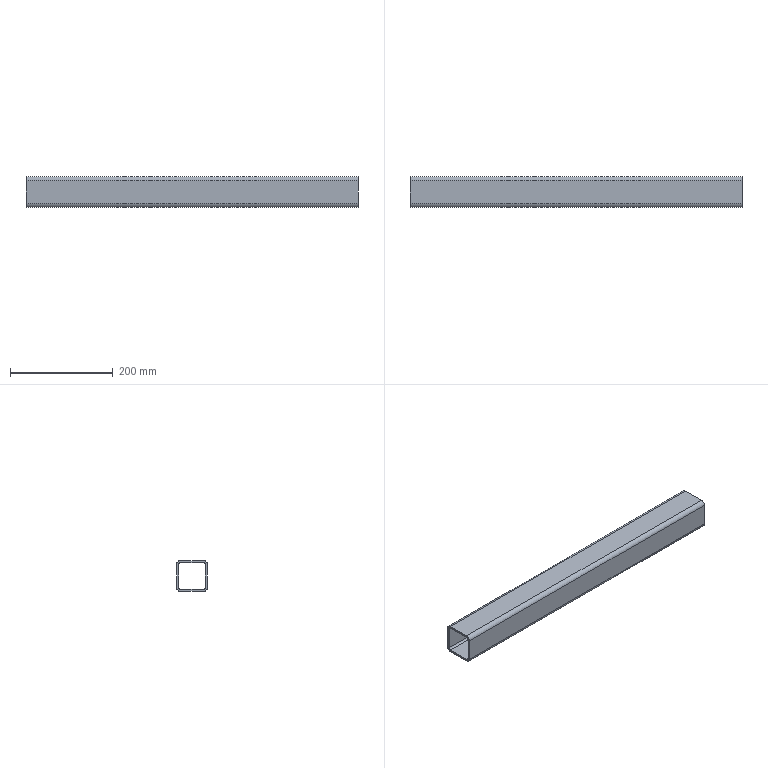Part | SolidWorks | features BaseBody 1 | 1 solid | 18 faces | box 645 x 60 x 60 mm | volume 551344 mm3 | plane 10 | cylinder 8 | commonest cylinder face diameters 8 x4 16 x4
STEP:
#1=CARTESIAN_POINT('',(700.,2488.,-1292.));
#2=VERTEX_POINT('',#1);
#3=CARTESIAN_POINT('',(700.,2488.,-1248.));
#4=VERTEX_POINT('',#3);
#5=CARTESIAN_POINT('',(700.,2488.,-1292.));
#6=DIRECTION('',(0.,0.,1.));
#7=VECTOR('',#6,1000.);
#8=LINE('',#5,#7);
#9=EDGE_CURVE('',#2,#4,#8,.T.);
#10=ORIENTED_EDGE('',*,*,#9,.T.);
#11=CARTESIAN_POINT('',(55.,2488.,-1248.));
#12=VERTEX_POINT('',#11);
#13=CARTESIAN_POINT('',(25.,2488.,-1248.));
#14=DIRECTION('',(-1.,0.,0.));
#15=VECTOR('',#14,1000.);
#16=LINE('',#13,#15);
#17=EDGE_CURVE('',#4,#12,#16,.T.);
#18=ORIENTED_EDGE('',*,*,#17,.T.);
#19=CARTESIAN_POINT('',(55.,2488.,-1292.));
#20=VERTEX_POINT('',#19);
#21=CARTESIAN_POINT('',(55.,2488.,-1292.));
#22=DIRECTION('',(0.,0.,-1.));
#23=VECTOR('',#22,1000.);
#24=LINE('',#21,#23);
#25=EDGE_CURVE('',#12,#20,#24,.T.);
#26=ORIENTED_EDGE('',*,*,#25,.T.);
#27=CARTESIAN_POINT('',(25.,2488.,-1292.));
#28=DIRECTION('',(1.,0.,0.));
#29=VECTOR('',#28,1000.);
#30=LINE('',#27,#29);
#31=EDGE_CURVE('',#20,#2,#30,.T.);
#32=ORIENTED_EDGE('',*,*,#31,.T.);
#33=EDGE_LOOP('',(#10,#18,#26,#32));
#34=FACE_OUTER_BOUND('',#33,.T.);
#35=CARTESIAN_POINT('',(25.,2488.,-1292.));
#36=DIRECTION('',(0.,-1.,0.));
#37=DIRECTION('',(0.,0.,-1.));
#38=AXIS2_PLACEMENT_3D('',#35,#36,#37);
#39=PLANE('',#38);
#40=ADVANCED_FACE('',(#34),#39,.T.);
#41=ORIENTED_EDGE('',*,*,#17,.F.);
#42=CARTESIAN_POINT('',(700.,2484.,-1244.));
#43=VERTEX_POINT('',#42);
#44=CARTESIAN_POINT('',(700.,2484.,-1248.));
#45=DIRECTION('',(-1.,0.,0.));
#46=DIRECTION('',(0.,0.,-1.));
#47=AXIS2_PLACEMENT_3D('',#44,#45,#46);
#48=CIRCLE('',#47,4.);
#49=EDGE_CURVE('',#43,#4,#48,.T.);
#50=ORIENTED_EDGE('',*,*,#49,.F.);
#51=CARTESIAN_POINT('',(55.,2484.,-1244.));
#52=VERTEX_POINT('',#51);
#53=CARTESIAN_POINT('',(25.,2484.,-1244.));
#54=DIRECTION('',(1.,0.,0.));
#55=VECTOR('',#54,1000.);
#56=LINE('',#53,#55);
#57=EDGE_CURVE('',#52,#43,#56,.T.);
#58=ORIENTED_EDGE('',*,*,#57,.F.);
#59=CARTESIAN_POINT('',(55.,2484.,-1248.));
#60=DIRECTION('',(1.,0.,0.));
#61=DIRECTION('',(0.,0.,-1.));
#62=AXIS2_PLACEMENT_3D('',#59,#60,#61);
#63=CIRCLE('',#62,4.);
#64=EDGE_CURVE('',#12,#52,#63,.T.);
#65=ORIENTED_EDGE('',*,*,#64,.F.);
#66=EDGE_LOOP('',(#41,#50,#58,#65));
#67=FACE_OUTER_BOUND('',#66,.T.);
#68=CARTESIAN_POINT('',(25.,2484.,-1248.));
#69=DIRECTION('',(1.,0.,0.));
#70=DIRECTION('',(0.,0.,-1.));
#71=AXIS2_PLACEMENT_3D('',#68,#69,#70);
#72=CYLINDRICAL_SURFACE('',#71,4.);
#73=ADVANCED_FACE('',(#67),#72,.F.);
#74=CARTESIAN_POINT('',(700.,2440.,-1244.));
#75=VERTEX_POINT('',#74);
#76=CARTESIAN_POINT('',(700.,2462.,-1244.));
#77=DIRECTION('',(0.,1.,0.));
#78=VECTOR('',#77,1000.);
#79=LINE('',#76,#78);
#80=EDGE_CURVE('',#75,#43,#79,.T.);
#81=ORIENTED_EDGE('',*,*,#80,.T.);
#82=ORIENTED_EDGE('',*,*,#49,.T.);
#83=ORIENTED_EDGE('',*,*,#9,.F.);
#84=CARTESIAN_POINT('',(700.,2484.,-1296.));
#85=VERTEX_POINT('',#84);
#86=CARTESIAN_POINT('',(700.,2484.,-1292.));
#87=DIRECTION('',(-1.,0.,0.));
#88=DIRECTION('',(0.,0.,-1.));
#89=AXIS2_PLACEMENT_3D('',#86,#87,#88);
#90=CIRCLE('',#89,4.);
#91=EDGE_CURVE('',#2,#85,#90,.T.);
#92=ORIENTED_EDGE('',*,*,#91,.T.);
#93=CARTESIAN_POINT('',(700.,2440.,-1296.));
#94=VERTEX_POINT('',#93);
#95=CARTESIAN_POINT('',(700.,2462.,-1296.));
#96=DIRECTION('',(0.,-1.,0.));
#97=VECTOR('',#96,1000.);
#98=LINE('',#95,#97);
#99=EDGE_CURVE('',#85,#94,#98,.T.);
#100=ORIENTED_EDGE('',*,*,#99,.T.);
#101=CARTESIAN_POINT('',(700.,2436.,-1292.));
#102=VERTEX_POINT('',#101);
#103=CARTESIAN_POINT('',(700.,2440.,-1292.));
#104=DIRECTION('',(-1.,0.,0.));
#105=DIRECTION('',(0.,0.,-1.));
#106=AXIS2_PLACEMENT_3D('',#103,#104,#105);
#107=CIRCLE('',#106,4.);
#108=EDGE_CURVE('',#94,#102,#107,.T.);
#109=ORIENTED_EDGE('',*,*,#108,.T.);
#110=CARTESIAN_POINT('',(700.,2436.,-1248.));
#111=VERTEX_POINT('',#110);
#112=CARTESIAN_POINT('',(700.,2436.,-1300.));
#113=DIRECTION('',(0.,0.,1.));
#114=VECTOR('',#113,1000.);
#115=LINE('',#112,#114);
#116=EDGE_CURVE('',#102,#111,#115,.T.);
#117=ORIENTED_EDGE('',*,*,#116,.T.);
#118=CARTESIAN_POINT('',(700.,2440.,-1248.));
#119=DIRECTION('',(-1.,0.,0.));
#120=DIRECTION('',(0.,0.,-1.));
#121=AXIS2_PLACEMENT_3D('',#118,#119,#120);
#122=CIRCLE('',#121,4.);
#123=EDGE_CURVE('',#111,#75,#122,.T.);
#124=ORIENTED_EDGE('',*,*,#123,.T.);
#125=EDGE_LOOP('',(#81,#82,#83,#92,#100,#109,#117,#124));
#126=FACE_BOUND('',#125,.T.);
#127=CARTESIAN_POINT('',(700.,2492.,-1248.));
#128=VERTEX_POINT('',#127);
#129=CARTESIAN_POINT('',(700.,2484.,-1240.));
#130=VERTEX_POINT('',#129);
#131=CARTESIAN_POINT('',(700.,2484.,-1248.));
#132=DIRECTION('',(1.,0.,0.));
#133=DIRECTION('',(0.,0.,-1.));
#134=AXIS2_PLACEMENT_3D('',#131,#132,#133);
#135=CIRCLE('',#134,8.);
#136=EDGE_CURVE('',#128,#130,#135,.T.);
#137=ORIENTED_EDGE('',*,*,#136,.T.);
#138=CARTESIAN_POINT('',(700.,2440.,-1240.));
#139=VERTEX_POINT('',#138);
#140=CARTESIAN_POINT('',(700.,2462.,-1240.));
#141=DIRECTION('',(0.,-1.,0.));
#142=VECTOR('',#141,1000.);
#143=LINE('',#140,#142);
#144=EDGE_CURVE('',#130,#139,#143,.T.);
#145=ORIENTED_EDGE('',*,*,#144,.T.);
#146=CARTESIAN_POINT('',(700.,2432.,-1248.));
#147=VERTEX_POINT('',#146);
#148=CARTESIAN_POINT('',(700.,2440.,-1248.));
#149=DIRECTION('',(1.,0.,0.));
#150=DIRECTION('',(0.,0.,-1.));
#151=AXIS2_PLACEMENT_3D('',#148,#149,#150);
#152=CIRCLE('',#151,8.);
#153=EDGE_CURVE('',#139,#147,#152,.T.);
#154=ORIENTED_EDGE('',*,*,#153,.T.);
#155=CARTESIAN_POINT('',(700.,2432.,-1292.));
#156=VERTEX_POINT('',#155);
#157=CARTESIAN_POINT('',(700.,2432.,-1300.));
#158=DIRECTION('',(0.,0.,-1.));
#159=VECTOR('',#158,1000.);
#160=LINE('',#157,#159);
#161=EDGE_CURVE('',#147,#156,#160,.T.);
#162=ORIENTED_EDGE('',*,*,#161,.T.);
#163=CARTESIAN_POINT('',(700.,2440.,-1300.));
#164=VERTEX_POINT('',#163);
#165=CARTESIAN_POINT('',(700.,2440.,-1292.));
#166=DIRECTION('',(1.,0.,0.));
#167=DIRECTION('',(0.,0.,-1.));
#168=AXIS2_PLACEMENT_3D('',#165,#166,#167);
#169=CIRCLE('',#168,8.);
#170=EDGE_CURVE('',#156,#164,#169,.T.);
#171=ORIENTED_EDGE('',*,*,#170,.T.);
#172=CARTESIAN_POINT('',(700.,2484.,-1300.));
#173=VERTEX_POINT('',#172);
#174=CARTESIAN_POINT('',(700.,2462.,-1300.));
#175=DIRECTION('',(0.,1.,0.));
#176=VECTOR('',#175,1000.);
#177=LINE('',#174,#176);
#178=EDGE_CURVE('',#164,#173,#177,.T.);
#179=ORIENTED_EDGE('',*,*,#178,.T.);
#180=CARTESIAN_POINT('',(700.,2492.,-1292.));
#181=VERTEX_POINT('',#180);
#182=CARTESIAN_POINT('',(700.,2484.,-1292.));
#183=DIRECTION('',(1.,0.,0.));
#184=DIRECTION('',(0.,0.,-1.));
#185=AXIS2_PLACEMENT_3D('',#182,#183,#184);
#186=CIRCLE('',#185,8.);
#187=EDGE_CURVE('',#173,#181,#186,.T.);
#188=ORIENTED_EDGE('',*,*,#187,.T.);
#189=CARTESIAN_POINT('',(700.,2492.,-1300.));
#190=DIRECTION('',(0.,0.,1.));
#191=VECTOR('',#190,1000.);
#192=LINE('',#189,#191);
#193=EDGE_CURVE('',#181,#128,#192,.T.);
#194=ORIENTED_EDGE('',*,*,#193,.T.);
#195=EDGE_LOOP('',(#137,#145,#154,#162,#171,#179,#188,#194));
#196=FACE_OUTER_BOUND('',#195,.T.);
#197=CARTESIAN_POINT('',(700.,2462.,-1300.));
#198=DIRECTION('',(1.,0.,0.));
#199=DIRECTION('',(0.,0.,-1.));
#200=AXIS2_PLACEMENT_3D('',#197,#198,#199);
#201=PLANE('',#200);
#202=ADVANCED_FACE('',(#126,#196),#201,.T.);
#203=CARTESIAN_POINT('',(55.,2484.,-1296.));
#204=VERTEX_POINT('',#203);
#205=CARTESIAN_POINT('',(25.,2484.,-1296.));
#206=DIRECTION('',(-1.,0.,0.));
#207=VECTOR('',#206,1000.);
#208=LINE('',#205,#207);
#209=EDGE_CURVE('',#85,#204,#208,.T.);
#210=ORIENTED_EDGE('',*,*,#209,.F.);
#211=ORIENTED_EDGE('',*,*,#91,.F.);
#212=ORIENTED_EDGE('',*,*,#31,.F.);
#213=CARTESIAN_POINT('',(55.,2484.,-1292.));
#214=DIRECTION('',(1.,0.,0.));
#215=DIRECTION('',(0.,0.,-1.));
#216=AXIS2_PLACEMENT_3D('',#213,#214,#215);
#217=CIRCLE('',#216,4.);
#218=EDGE_CURVE('',#204,#20,#217,.T.);
#219=ORIENTED_EDGE('',*,*,#218,.F.);
#220=EDGE_LOOP('',(#210,#211,#212,#219));
#221=FACE_OUTER_BOUND('',#220,.T.);
#222=CARTESIAN_POINT('',(25.,2484.,-1292.));
#223=DIRECTION('',(1.,0.,0.));
#224=DIRECTION('',(0.,0.,-1.));
#225=AXIS2_PLACEMENT_3D('',#222,#223,#224);
#226=CYLINDRICAL_SURFACE('',#225,4.);
#227=ADVANCED_FACE('',(#221),#226,.F.);
#228=ORIENTED_EDGE('',*,*,#64,.T.);
#229=CARTESIAN_POINT('',(55.,2440.,-1244.));
#230=VERTEX_POINT('',#229);
#231=CARTESIAN_POINT('',(55.,2484.,-1244.));
#232=DIRECTION('',(0.,-1.,0.));
#233=VECTOR('',#232,1000.);
#234=LINE('',#231,#233);
#235=EDGE_CURVE('',#52,#230,#234,.T.);
#236=ORIENTED_EDGE('',*,*,#235,.T.);
#237=CARTESIAN_POINT('',(55.,2436.,-1248.));
#238=VERTEX_POINT('',#237);
#239=CARTESIAN_POINT('',(55.,2440.,-1248.));
#240=DIRECTION('',(1.,0.,0.));
#241=DIRECTION('',(0.,0.,-1.));
#242=AXIS2_PLACEMENT_3D('',#239,#240,#241);
#243=CIRCLE('',#242,4.);
#244=EDGE_CURVE('',#230,#238,#243,.T.);
#245=ORIENTED_EDGE('',*,*,#244,.T.);
#246=CARTESIAN_POINT('',(55.,2436.,-1292.));
#247=VERTEX_POINT('',#246);
#248=CARTESIAN_POINT('',(55.,2436.,-1270.));
#249=DIRECTION('',(0.,0.,-1.));
#250=VECTOR('',#249,1000.);
#251=LINE('',#248,#250);
#252=EDGE_CURVE('',#238,#247,#251,.T.);
#253=ORIENTED_EDGE('',*,*,#252,.T.);
#254=CARTESIAN_POINT('',(55.,2440.,-1296.));
#255=VERTEX_POINT('',#254);
#256=CARTESIAN_POINT('',(55.,2440.,-1292.));
#257=DIRECTION('',(1.,0.,0.));
#258=DIRECTION('',(0.,0.,-1.));
#259=AXIS2_PLACEMENT_3D('',#256,#257,#258);
#260=CIRCLE('',#259,4.);
#261=EDGE_CURVE('',#247,#255,#260,.T.);
#262=ORIENTED_EDGE('',*,*,#261,.T.);
#263=CARTESIAN_POINT('',(55.,2484.,-1296.));
#264=DIRECTION('',(0.,1.,0.));
#265=VECTOR('',#264,1000.);
#266=LINE('',#263,#265);
#267=EDGE_CURVE('',#255,#204,#266,.T.);
#268=ORIENTED_EDGE('',*,*,#267,.T.);
#269=ORIENTED_EDGE('',*,*,#218,.T.);
#270=ORIENTED_EDGE('',*,*,#25,.F.);
#271=EDGE_LOOP('',(#228,#236,#245,#253,#262,#268,#269,#270));
#272=FACE_BOUND('',#271,.T.);
#273=CARTESIAN_POINT('',(55.,2432.,-1292.));
#274=VERTEX_POINT('',#273);
#275=CARTESIAN_POINT('',(55.,2432.,-1248.));
#276=VERTEX_POINT('',#275);
#277=CARTESIAN_POINT('',(55.,2432.,-1270.));
#278=DIRECTION('',(0.,0.,1.));
#279=VECTOR('',#278,1000.);
#280=LINE('',#277,#279);
#281=EDGE_CURVE('',#274,#276,#280,.T.);
#282=ORIENTED_EDGE('',*,*,#281,.T.);
#283=CARTESIAN_POINT('',(55.,2440.,-1240.));
#284=VERTEX_POINT('',#283);
#285=CARTESIAN_POINT('',(55.,2440.,-1248.));
#286=DIRECTION('',(-1.,0.,0.));
#287=DIRECTION('',(0.,0.,-1.));
#288=AXIS2_PLACEMENT_3D('',#285,#286,#287);
#289=CIRCLE('',#288,8.);
#290=EDGE_CURVE('',#276,#284,#289,.T.);
#291=ORIENTED_EDGE('',*,*,#290,.T.);
#292=CARTESIAN_POINT('',(55.,2484.,-1240.));
#293=VERTEX_POINT('',#292);
#294=CARTESIAN_POINT('',(55.,2484.,-1240.));
#295=DIRECTION('',(0.,1.,0.));
#296=VECTOR('',#295,1000.);
#297=LINE('',#294,#296);
#298=EDGE_CURVE('',#284,#293,#297,.T.);
#299=ORIENTED_EDGE('',*,*,#298,.T.);
#300=CARTESIAN_POINT('',(55.,2492.,-1248.));
#301=VERTEX_POINT('',#300);
#302=CARTESIAN_POINT('',(55.,2484.,-1248.));
#303=DIRECTION('',(-1.,0.,0.));
#304=DIRECTION('',(0.,0.,-1.));
#305=AXIS2_PLACEMENT_3D('',#302,#303,#304);
#306=CIRCLE('',#305,8.);
#307=EDGE_CURVE('',#293,#301,#306,.T.);
#308=ORIENTED_EDGE('',*,*,#307,.T.);
#309=CARTESIAN_POINT('',(55.,2492.,-1292.));
#310=VERTEX_POINT('',#309);
#311=CARTESIAN_POINT('',(55.,2492.,-1270.));
#312=DIRECTION('',(0.,0.,-1.));
#313=VECTOR('',#312,1000.);
#314=LINE('',#311,#313);
#315=EDGE_CURVE('',#301,#310,#314,.T.);
#316=ORIENTED_EDGE('',*,*,#315,.T.);
#317=CARTESIAN_POINT('',(55.,2484.,-1300.));
#318=VERTEX_POINT('',#317);
#319=CARTESIAN_POINT('',(55.,2484.,-1292.));
#320=DIRECTION('',(-1.,0.,0.));
#321=DIRECTION('',(0.,0.,-1.));
#322=AXIS2_PLACEMENT_3D('',#319,#320,#321);
#323=CIRCLE('',#322,8.);
#324=EDGE_CURVE('',#310,#318,#323,.T.);
#325=ORIENTED_EDGE('',*,*,#324,.T.);
#326=CARTESIAN_POINT('',(55.,2440.,-1300.));
#327=VERTEX_POINT('',#326);
#328=CARTESIAN_POINT('',(55.,2484.,-1300.));
#329=DIRECTION('',(0.,-1.,0.));
#330=VECTOR('',#329,1000.);
#331=LINE('',#328,#330);
#332=EDGE_CURVE('',#318,#327,#331,.T.);
#333=ORIENTED_EDGE('',*,*,#332,.T.);
#334=CARTESIAN_POINT('',(55.,2440.,-1292.));
#335=DIRECTION('',(-1.,0.,0.));
#336=DIRECTION('',(0.,0.,-1.));
#337=AXIS2_PLACEMENT_3D('',#334,#335,#336);
#338=CIRCLE('',#337,8.);
#339=EDGE_CURVE('',#327,#274,#338,.T.);
#340=ORIENTED_EDGE('',*,*,#339,.T.);
#341=EDGE_LOOP('',(#282,#291,#299,#308,#316,#325,#333,#340));
#342=FACE_OUTER_BOUND('',#341,.T.);
#343=CARTESIAN_POINT('',(55.,2484.,-1270.));
#344=DIRECTION('',(-1.,0.,0.));
#345=DIRECTION('',(0.,0.,1.));
#346=AXIS2_PLACEMENT_3D('',#343,#344,#345);
#347=PLANE('',#346);
#348=ADVANCED_FACE('',(#272,#342),#347,.T.);
#349=ORIENTED_EDGE('',*,*,#80,.F.);
#350=CARTESIAN_POINT('',(25.,2440.,-1244.));
#351=DIRECTION('',(-1.,0.,0.));
#352=VECTOR('',#351,1000.);
#353=LINE('',#350,#352);
#354=EDGE_CURVE('',#75,#230,#353,.T.);
#355=ORIENTED_EDGE('',*,*,#354,.T.);
#356=ORIENTED_EDGE('',*,*,#235,.F.);
#357=ORIENTED_EDGE('',*,*,#57,.T.);
#358=EDGE_LOOP('',(#349,#355,#356,#357));
#359=FACE_OUTER_BOUND('',#358,.T.);
#360=CARTESIAN_POINT('',(25.,2440.,-1244.));
#361=DIRECTION('',(0.,0.,-1.));
#362=DIRECTION('',(-1.,0.,0.));
#363=AXIS2_PLACEMENT_3D('',#360,#361,#362);
#364=PLANE('',#363);
#365=ADVANCED_FACE('',(#359),#364,.T.);
#366=ORIENTED_EDGE('',*,*,#354,.F.);
#367=ORIENTED_EDGE('',*,*,#123,.F.);
#368=CARTESIAN_POINT('',(25.,2436.,-1248.));
#369=DIRECTION('',(1.,0.,0.));
#370=VECTOR('',#369,1000.);
#371=LINE('',#368,#370);
#372=EDGE_CURVE('',#238,#111,#371,.T.);
#373=ORIENTED_EDGE('',*,*,#372,.F.);
#374=ORIENTED_EDGE('',*,*,#244,.F.);
#375=EDGE_LOOP('',(#366,#367,#373,#374));
#376=FACE_OUTER_BOUND('',#375,.T.);
#377=CARTESIAN_POINT('',(25.,2440.,-1248.));
#378=DIRECTION('',(1.,0.,0.));
#379=DIRECTION('',(0.,0.,-1.));
#380=AXIS2_PLACEMENT_3D('',#377,#378,#379);
#381=CYLINDRICAL_SURFACE('',#380,4.);
#382=ADVANCED_FACE('',(#376),#381,.F.);
#383=ORIENTED_EDGE('',*,*,#116,.F.);
#384=CARTESIAN_POINT('',(25.,2436.,-1292.));
#385=DIRECTION('',(-1.,0.,0.));
#386=VECTOR('',#385,1000.);
#387=LINE('',#384,#386);
#388=EDGE_CURVE('',#102,#247,#387,.T.);
#389=ORIENTED_EDGE('',*,*,#388,.T.);
#390=ORIENTED_EDGE('',*,*,#252,.F.);
#391=ORIENTED_EDGE('',*,*,#372,.T.);
#392=EDGE_LOOP('',(#383,#389,#390,#391));
#393=FACE_OUTER_BOUND('',#392,.T.);
#394=CARTESIAN_POINT('',(25.,2436.,-1248.));
#395=DIRECTION('',(0.,1.,0.));
#396=DIRECTION('',(0.,0.,1.));
#397=AXIS2_PLACEMENT_3D('',#394,#395,#396);
#398=PLANE('',#397);
#399=ADVANCED_FACE('',(#393),#398,.T.);
#400=ORIENTED_EDGE('',*,*,#388,.F.);
#401=ORIENTED_EDGE('',*,*,#108,.F.);
#402=CARTESIAN_POINT('',(25.,2440.,-1296.));
#403=DIRECTION('',(1.,0.,0.));
#404=VECTOR('',#403,1000.);
#405=LINE('',#402,#404);
#406=EDGE_CURVE('',#255,#94,#405,.T.);
#407=ORIENTED_EDGE('',*,*,#406,.F.);
#408=ORIENTED_EDGE('',*,*,#261,.F.);
#409=EDGE_LOOP('',(#400,#401,#407,#408));
#410=FACE_OUTER_BOUND('',#409,.T.);
#411=CARTESIAN_POINT('',(25.,2440.,-1292.));
#412=DIRECTION('',(1.,0.,0.));
#413=DIRECTION('',(0.,0.,-1.));
#414=AXIS2_PLACEMENT_3D('',#411,#412,#413);
#415=CYLINDRICAL_SURFACE('',#414,4.);
#416=ADVANCED_FACE('',(#410),#415,.F.);
#417=ORIENTED_EDGE('',*,*,#99,.F.);
#418=ORIENTED_EDGE('',*,*,#209,.T.);
#419=ORIENTED_EDGE('',*,*,#267,.F.);
#420=ORIENTED_EDGE('',*,*,#406,.T.);
#421=EDGE_LOOP('',(#417,#418,#419,#420));
#422=FACE_OUTER_BOUND('',#421,.T.);
#423=CARTESIAN_POINT('',(25.,2484.,-1296.));
#424=DIRECTION('',(0.,0.,1.));
#425=DIRECTION('',(1.,0.,0.));
#426=AXIS2_PLACEMENT_3D('',#423,#424,#425);
#427=PLANE('',#426);
#428=ADVANCED_FACE('',(#422),#427,.T.);
#429=ORIENTED_EDGE('',*,*,#144,.F.);
#430=CARTESIAN_POINT('',(25.,2484.,-1240.));
#431=DIRECTION('',(1.,0.,0.));
#432=VECTOR('',#431,1000.);
#433=LINE('',#430,#432);
#434=EDGE_CURVE('',#293,#130,#433,.T.);
#435=ORIENTED_EDGE('',*,*,#434,.F.);
#436=ORIENTED_EDGE('',*,*,#298,.F.);
#437=CARTESIAN_POINT('',(25.,2440.,-1240.));
#438=DIRECTION('',(-1.,0.,0.));
#439=VECTOR('',#438,1000.);
#440=LINE('',#437,#439);
#441=EDGE_CURVE('',#139,#284,#440,.T.);
#442=ORIENTED_EDGE('',*,*,#441,.F.);
#443=EDGE_LOOP('',(#429,#435,#436,#442));
#444=FACE_OUTER_BOUND('',#443,.T.);
#445=CARTESIAN_POINT('',(25.,2440.,-1240.));
#446=DIRECTION('',(0.,0.,-1.));
#447=DIRECTION('',(-1.,0.,0.));
#448=AXIS2_PLACEMENT_3D('',#445,#446,#447);
#449=PLANE('',#448);
#450=ADVANCED_FACE('',(#444),#449,.F.);
#451=CARTESIAN_POINT('',(25.,2492.,-1248.));
#452=DIRECTION('',(-1.,0.,0.));
#453=VECTOR('',#452,1000.);
#454=LINE('',#451,#453);
#455=EDGE_CURVE('',#128,#301,#454,.T.);
#456=ORIENTED_EDGE('',*,*,#455,.T.);
#457=ORIENTED_EDGE('',*,*,#307,.F.);
#458=ORIENTED_EDGE('',*,*,#434,.T.);
#459=ORIENTED_EDGE('',*,*,#136,.F.);
#460=EDGE_LOOP('',(#456,#457,#458,#459));
#461=FACE_OUTER_BOUND('',#460,.T.);
#462=CARTESIAN_POINT('',(25.,2484.,-1248.));
#463=DIRECTION('',(1.,0.,0.));
#464=DIRECTION('',(0.,0.,-1.));
#465=AXIS2_PLACEMENT_3D('',#462,#463,#464);
#466=CYLINDRICAL_SURFACE('',#465,8.);
#467=ADVANCED_FACE('',(#461),#466,.T.);
#468=ORIENTED_EDGE('',*,*,#193,.F.);
#469=CARTESIAN_POINT('',(25.,2492.,-1292.));
#470=DIRECTION('',(1.,0.,0.));
#471=VECTOR('',#470,1000.);
#472=LINE('',#469,#471);
#473=EDGE_CURVE('',#310,#181,#472,.T.);
#474=ORIENTED_EDGE('',*,*,#473,.F.);
#475=ORIENTED_EDGE('',*,*,#315,.F.);
#476=ORIENTED_EDGE('',*,*,#455,.F.);
#477=EDGE_LOOP('',(#468,#474,#475,#476));
#478=FACE_OUTER_BOUND('',#477,.T.);
#479=CARTESIAN_POINT('',(25.,2492.,-1292.));
#480=DIRECTION('',(0.,-1.,0.));
#481=DIRECTION('',(0.,0.,-1.));
#482=AXIS2_PLACEMENT_3D('',#479,#480,#481);
#483=PLANE('',#482);
#484=ADVANCED_FACE('',(#478),#483,.F.);
#485=CARTESIAN_POINT('',(25.,2484.,-1300.));
#486=DIRECTION('',(-1.,0.,0.));
#487=VECTOR('',#486,1000.);
#488=LINE('',#485,#487);
#489=EDGE_CURVE('',#173,#318,#488,.T.);
#490=ORIENTED_EDGE('',*,*,#489,.T.);
#491=ORIENTED_EDGE('',*,*,#324,.F.);
#492=ORIENTED_EDGE('',*,*,#473,.T.);
#493=ORIENTED_EDGE('',*,*,#187,.F.);
#494=EDGE_LOOP('',(#490,#491,#492,#493));
#495=FACE_OUTER_BOUND('',#494,.T.);
#496=CARTESIAN_POINT('',(25.,2484.,-1292.));
#497=DIRECTION('',(1.,0.,0.));
#498=DIRECTION('',(0.,0.,-1.));
#499=AXIS2_PLACEMENT_3D('',#496,#497,#498);
#500=CYLINDRICAL_SURFACE('',#499,8.);
#501=ADVANCED_FACE('',(#495),#500,.T.);
#502=ORIENTED_EDGE('',*,*,#178,.F.);
#503=CARTESIAN_POINT('',(25.,2440.,-1300.));
#504=DIRECTION('',(1.,0.,0.));
#505=VECTOR('',#504,1000.);
#506=LINE('',#503,#505);
#507=EDGE_CURVE('',#327,#164,#506,.T.);
#508=ORIENTED_EDGE('',*,*,#507,.F.);
#509=ORIENTED_EDGE('',*,*,#332,.F.);
#510=ORIENTED_EDGE('',*,*,#489,.F.);
#511=EDGE_LOOP('',(#502,#508,#509,#510));
#512=FACE_OUTER_BOUND('',#511,.T.);
#513=CARTESIAN_POINT('',(25.,2484.,-1300.));
#514=DIRECTION('',(0.,0.,1.));
#515=DIRECTION('',(1.,0.,0.));
#516=AXIS2_PLACEMENT_3D('',#513,#514,#515);
#517=PLANE('',#516);
#518=ADVANCED_FACE('',(#512),#517,.F.);
#519=CARTESIAN_POINT('',(25.,2432.,-1292.));
#520=DIRECTION('',(-1.,0.,0.));
#521=VECTOR('',#520,1000.);
#522=LINE('',#519,#521);
#523=EDGE_CURVE('',#156,#274,#522,.T.);
#524=ORIENTED_EDGE('',*,*,#523,.T.);
#525=ORIENTED_EDGE('',*,*,#339,.F.);
#526=ORIENTED_EDGE('',*,*,#507,.T.);
#527=ORIENTED_EDGE('',*,*,#170,.F.);
#528=EDGE_LOOP('',(#524,#525,#526,#527));
#529=FACE_OUTER_BOUND('',#528,.T.);
#530=CARTESIAN_POINT('',(25.,2440.,-1292.));
#531=DIRECTION('',(1.,0.,0.));
#532=DIRECTION('',(0.,0.,-1.));
#533=AXIS2_PLACEMENT_3D('',#530,#531,#532);
#534=CYLINDRICAL_SURFACE('',#533,8.);
#535=ADVANCED_FACE('',(#529),#534,.T.);
#536=ORIENTED_EDGE('',*,*,#161,.F.);
#537=CARTESIAN_POINT('',(25.,2432.,-1248.));
#538=DIRECTION('',(1.,0.,0.));
#539=VECTOR('',#538,1000.);
#540=LINE('',#537,#539);
#541=EDGE_CURVE('',#276,#147,#540,.T.);
#542=ORIENTED_EDGE('',*,*,#541,.F.);
#543=ORIENTED_EDGE('',*,*,#281,.F.);
#544=ORIENTED_EDGE('',*,*,#523,.F.);
#545=EDGE_LOOP('',(#536,#542,#543,#544));
#546=FACE_OUTER_BOUND('',#545,.T.);
#547=CARTESIAN_POINT('',(25.,2432.,-1248.));
#548=DIRECTION('',(0.,1.,0.));
#549=DIRECTION('',(0.,0.,1.));
#550=AXIS2_PLACEMENT_3D('',#547,#548,#549);
#551=PLANE('',#550);
#552=ADVANCED_FACE('',(#546),#551,.F.);
#553=ORIENTED_EDGE('',*,*,#441,.T.);
#554=ORIENTED_EDGE('',*,*,#290,.F.);
#555=ORIENTED_EDGE('',*,*,#541,.T.);
#556=ORIENTED_EDGE('',*,*,#153,.F.);
#557=EDGE_LOOP('',(#553,#554,#555,#556));
#558=FACE_OUTER_BOUND('',#557,.T.);
#559=CARTESIAN_POINT('',(25.,2440.,-1248.));
#560=DIRECTION('',(1.,0.,0.));
#561=DIRECTION('',(0.,0.,-1.));
#562=AXIS2_PLACEMENT_3D('',#559,#560,#561);
#563=CYLINDRICAL_SURFACE('',#562,8.);
#564=ADVANCED_FACE('',(#558),#563,.T.);
#565=CLOSED_SHELL('',(#40,#73,#202,#227,#348,#365,#382,#399,#416,#428,#450,#467,#484,#501,#518,#535,#552,#564));
#566=MANIFOLD_SOLID_BREP('',#565);
#567=CARTESIAN_POINT('',(0.,0.,0.));
#568=DIRECTION('',(0.,0.,1.));
#569=DIRECTION('',(1.,0.,0.));
#570=AXIS2_PLACEMENT_3D('',#567,#568,#569);
#571=(LENGTH_UNIT()NAMED_UNIT(*)SI_UNIT(.MILLI.,.METRE.));
#572=UNCERTAINTY_MEASURE_WITH_UNIT(LENGTH_MEASURE(0.00001),#571,'','');
#573=(NAMED_UNIT(*)PLANE_ANGLE_UNIT()SI_UNIT($,.RADIAN.));
#574=(NAMED_UNIT(*)SI_UNIT($,.STERADIAN.)SOLID_ANGLE_UNIT());
#575=(GEOMETRIC_REPRESENTATION_CONTEXT(3)GLOBAL_UNCERTAINTY_ASSIGNED_CONTEXT((#572))GLOBAL_UNIT_ASSIGNED_CONTEXT((#571,#573,#574))REPRESENTATION_CONTEXT('',''));
#576=ADVANCED_BREP_SHAPE_REPRESENTATION('',(#566,#570),#575);